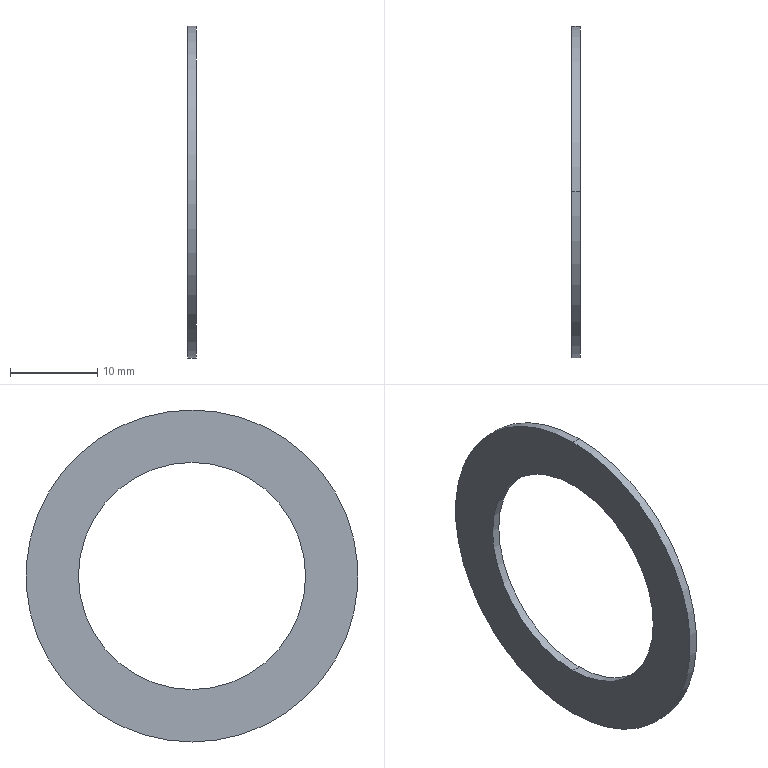Part | STEP file | 1 solid | 6 faces | box 1 x 38 x 38 mm | volume 603.186 mm3 | cylinder 4 | plane 2 | commonest cylinder face diameters 26 x2 38 x2
STEP:
#1=CARTESIAN_POINT('',(0.,0.,0.));
#2=DIRECTION('',(0.,0.,1.));
#3=DIRECTION('',(1.,0.,0.));
#4=AXIS2_PLACEMENT_3D('',#1,#2,#3);
#5=CARTESIAN_POINT('',(0.,0.,-13.));
#6=VERTEX_POINT('',#5);
#7=CARTESIAN_POINT('',(1.,0.,-13.));
#8=VERTEX_POINT('',#7);
#9=CARTESIAN_POINT('',(0.5,0.,-13.));
#10=DIRECTION('',(1.,0.,0.));
#11=VECTOR('',#10,1.);
#12=LINE('',#9,#11);
#13=CARTESIAN_POINT('',(0.5,0.,0.));
#14=DIRECTION('',(1.,0.,0.));
#15=DIRECTION('',(0.,0.,-1.));
#16=AXIS2_PLACEMENT_3D('',#13,#14,#15);
#17=CYLINDRICAL_SURFACE('',#16,13.);
#18=CARTESIAN_POINT('',(6.283,0.));
#19=DIRECTION('',(0.,1.));
#20=VECTOR('',#19,1.);
#21=LINE('',#18,#20);
#22=(GEOMETRIC_REPRESENTATION_CONTEXT(2)PARAMETRIC_REPRESENTATION_CONTEXT()REPRESENTATION_CONTEXT('',''));
#23=DEFINITIONAL_REPRESENTATION('',(#21),#22);
#24=PCURVE('',#17,#23);
#25=CARTESIAN_POINT('',(0.5,0.,0.));
#26=DIRECTION('',(1.,0.,0.));
#27=DIRECTION('',(0.,0.,-1.));
#28=AXIS2_PLACEMENT_3D('',#25,#26,#27);
#29=CYLINDRICAL_SURFACE('',#28,13.);
#30=CARTESIAN_POINT('',(0.,0.));
#31=DIRECTION('',(0.,1.));
#32=VECTOR('',#31,1.);
#33=LINE('',#30,#32);
#34=(GEOMETRIC_REPRESENTATION_CONTEXT(2)PARAMETRIC_REPRESENTATION_CONTEXT()REPRESENTATION_CONTEXT('',''));
#35=DEFINITIONAL_REPRESENTATION('',(#33),#34);
#36=PCURVE('',#29,#35);
#37=SURFACE_CURVE('',#12,(#24,#36),.PCURVE_S1.);
#38=EDGE_CURVE('',#6,#8,#37,.T.);
#39=ORIENTED_EDGE('',*,*,#38,.T.);
#40=CARTESIAN_POINT('',(1.,0.,13.));
#41=VERTEX_POINT('',#40);
#42=CARTESIAN_POINT('',(1.,0.,0.));
#43=DIRECTION('',(-1.,0.,0.));
#44=DIRECTION('',(0.,0.,-1.));
#45=AXIS2_PLACEMENT_3D('',#42,#43,#44);
#46=CIRCLE('',#45,13.);
#47=CARTESIAN_POINT('',(6.283,0.5));
#48=DIRECTION('',(-1.,0.));
#49=VECTOR('',#48,1.);
#50=LINE('',#47,#49);
#51=(GEOMETRIC_REPRESENTATION_CONTEXT(2)PARAMETRIC_REPRESENTATION_CONTEXT()REPRESENTATION_CONTEXT('',''));
#52=DEFINITIONAL_REPRESENTATION('',(#50),#51);
#53=PCURVE('',#17,#52);
#54=CARTESIAN_POINT('',(1.,16.,0.));
#55=DIRECTION('',(1.,0.,0.));
#56=DIRECTION('',(0.,0.,-1.));
#57=AXIS2_PLACEMENT_3D('',#54,#55,#56);
#58=PLANE('',#57);
#59=CARTESIAN_POINT('',(13.,-16.));
#60=CARTESIAN_POINT('',(13.,-38.517));
#61=CARTESIAN_POINT('',(-6.5,-27.258));
#62=CARTESIAN_POINT('',(-26.,-16.));
#63=CARTESIAN_POINT('',(-6.5,-4.742));
#64=CARTESIAN_POINT('',(13.,6.517));
#65=CARTESIAN_POINT('',(13.,-16.));
#66=(BOUNDED_CURVE()B_SPLINE_CURVE(2,(#59,#60,#61,#62,#63,#64,#65),.UNSPECIFIED.,.T.,.F.)B_SPLINE_CURVE_WITH_KNOTS((1,2,2,2,2,1),(-2.094,0.,2.094,4.189,6.283,8.378),.UNSPECIFIED.)CURVE()GEOMETRIC_REPRESENTATION_ITEM()RATIONAL_B_SPLINE_CURVE((1.,0.5,1.,0.5,1.,0.5,1.))REPRESENTATION_ITEM(''));
#67=(GEOMETRIC_REPRESENTATION_CONTEXT(2)PARAMETRIC_REPRESENTATION_CONTEXT()REPRESENTATION_CONTEXT('',''));
#68=DEFINITIONAL_REPRESENTATION('',(#66),#67);
#69=PCURVE('',#58,#68);
#70=SURFACE_CURVE('',#46,(#53,#69),.PCURVE_S1.);
#71=EDGE_CURVE('',#8,#41,#70,.T.);
#72=ORIENTED_EDGE('',*,*,#71,.T.);
#73=CARTESIAN_POINT('',(0.,0.,13.));
#74=VERTEX_POINT('',#73);
#75=CARTESIAN_POINT('',(0.5,0.,13.));
#76=DIRECTION('',(1.,0.,0.));
#77=VECTOR('',#76,1.);
#78=LINE('',#75,#77);
#79=CARTESIAN_POINT('',(3.142,0.));
#80=DIRECTION('',(0.,1.));
#81=VECTOR('',#80,1.);
#82=LINE('',#79,#81);
#83=(GEOMETRIC_REPRESENTATION_CONTEXT(2)PARAMETRIC_REPRESENTATION_CONTEXT()REPRESENTATION_CONTEXT('',''));
#84=DEFINITIONAL_REPRESENTATION('',(#82),#83);
#85=PCURVE('',#17,#84);
#86=CARTESIAN_POINT('',(3.142,0.));
#87=DIRECTION('',(0.,1.));
#88=VECTOR('',#87,1.);
#89=LINE('',#86,#88);
#90=(GEOMETRIC_REPRESENTATION_CONTEXT(2)PARAMETRIC_REPRESENTATION_CONTEXT()REPRESENTATION_CONTEXT('',''));
#91=DEFINITIONAL_REPRESENTATION('',(#89),#90);
#92=PCURVE('',#29,#91);
#93=SURFACE_CURVE('',#78,(#85,#92),.PCURVE_S1.);
#94=EDGE_CURVE('',#74,#41,#93,.T.);
#95=ORIENTED_EDGE('',*,*,#94,.F.);
#96=CARTESIAN_POINT('',(0.,0.,0.));
#97=DIRECTION('',(1.,0.,0.));
#98=DIRECTION('',(0.,0.,-1.));
#99=AXIS2_PLACEMENT_3D('',#96,#97,#98);
#100=CIRCLE('',#99,13.);
#101=CARTESIAN_POINT('',(0.,-0.5));
#102=DIRECTION('',(1.,0.));
#103=VECTOR('',#102,1.);
#104=LINE('',#101,#103);
#105=(GEOMETRIC_REPRESENTATION_CONTEXT(2)PARAMETRIC_REPRESENTATION_CONTEXT()REPRESENTATION_CONTEXT('',''));
#106=DEFINITIONAL_REPRESENTATION('',(#104),#105);
#107=PCURVE('',#17,#106);
#108=CARTESIAN_POINT('',(0.,16.,0.));
#109=DIRECTION('',(-1.,0.,0.));
#110=DIRECTION('',(0.,0.,1.));
#111=AXIS2_PLACEMENT_3D('',#108,#109,#110);
#112=PLANE('',#111);
#113=CARTESIAN_POINT('',(-13.,-16.));
#114=CARTESIAN_POINT('',(-13.,6.517));
#115=CARTESIAN_POINT('',(6.5,-4.742));
#116=CARTESIAN_POINT('',(26.,-16.));
#117=CARTESIAN_POINT('',(6.5,-27.258));
#118=CARTESIAN_POINT('',(-13.,-38.517));
#119=CARTESIAN_POINT('',(-13.,-16.));
#120=(BOUNDED_CURVE()B_SPLINE_CURVE(2,(#113,#114,#115,#116,#117,#118,#119),.UNSPECIFIED.,.T.,.F.)B_SPLINE_CURVE_WITH_KNOTS((1,2,2,2,2,1),(-2.094,0.,2.094,4.189,6.283,8.378),.UNSPECIFIED.)CURVE()GEOMETRIC_REPRESENTATION_ITEM()RATIONAL_B_SPLINE_CURVE((1.,0.5,1.,0.5,1.,0.5,1.))REPRESENTATION_ITEM(''));
#121=(GEOMETRIC_REPRESENTATION_CONTEXT(2)PARAMETRIC_REPRESENTATION_CONTEXT()REPRESENTATION_CONTEXT('',''));
#122=DEFINITIONAL_REPRESENTATION('',(#120),#121);
#123=PCURVE('',#112,#122);
#124=SURFACE_CURVE('',#100,(#107,#123),.PCURVE_S1.);
#125=EDGE_CURVE('',#74,#6,#124,.T.);
#126=ORIENTED_EDGE('',*,*,#125,.T.);
#127=EDGE_LOOP('',(#39,#72,#95,#126));
#128=FACE_BOUND('',#127,.F.);
#129=ADVANCED_FACE('',(#128),#17,.F.);
#130=CARTESIAN_POINT('',(0.,0.,-19.));
#131=VERTEX_POINT('',#130);
#132=CARTESIAN_POINT('',(0.,0.,19.));
#133=VERTEX_POINT('',#132);
#134=CARTESIAN_POINT('',(0.,0.,0.));
#135=DIRECTION('',(1.,0.,0.));
#136=DIRECTION('',(0.,0.,-1.));
#137=AXIS2_PLACEMENT_3D('',#134,#135,#136);
#138=CIRCLE('',#137,19.);
#139=CARTESIAN_POINT('',(0.5,0.,0.));
#140=DIRECTION('',(1.,0.,0.));
#141=DIRECTION('',(0.,0.,-1.));
#142=AXIS2_PLACEMENT_3D('',#139,#140,#141);
#143=CYLINDRICAL_SURFACE('',#142,19.);
#144=CARTESIAN_POINT('',(0.,-0.5));
#145=DIRECTION('',(1.,0.));
#146=VECTOR('',#145,1.);
#147=LINE('',#144,#146);
#148=(GEOMETRIC_REPRESENTATION_CONTEXT(2)PARAMETRIC_REPRESENTATION_CONTEXT()REPRESENTATION_CONTEXT('',''));
#149=DEFINITIONAL_REPRESENTATION('',(#147),#148);
#150=PCURVE('',#143,#149);
#151=CARTESIAN_POINT('',(-19.,-16.));
#152=CARTESIAN_POINT('',(-19.,16.909));
#153=CARTESIAN_POINT('',(9.5,0.4545));
#154=CARTESIAN_POINT('',(38.,-16.));
#155=CARTESIAN_POINT('',(9.5,-32.454));
#156=CARTESIAN_POINT('',(-19.,-48.909));
#157=CARTESIAN_POINT('',(-19.,-16.));
#158=(BOUNDED_CURVE()B_SPLINE_CURVE(2,(#151,#152,#153,#154,#155,#156,#157),.UNSPECIFIED.,.T.,.F.)B_SPLINE_CURVE_WITH_KNOTS((1,2,2,2,2,1),(-2.094,0.,2.094,4.189,6.283,8.378),.UNSPECIFIED.)CURVE()GEOMETRIC_REPRESENTATION_ITEM()RATIONAL_B_SPLINE_CURVE((1.,0.5,1.,0.5,1.,0.5,1.))REPRESENTATION_ITEM(''));
#159=(GEOMETRIC_REPRESENTATION_CONTEXT(2)PARAMETRIC_REPRESENTATION_CONTEXT()REPRESENTATION_CONTEXT('',''));
#160=DEFINITIONAL_REPRESENTATION('',(#158),#159);
#161=PCURVE('',#112,#160);
#162=SURFACE_CURVE('',#138,(#150,#161),.PCURVE_S1.);
#163=EDGE_CURVE('',#131,#133,#162,.T.);
#164=ORIENTED_EDGE('',*,*,#163,.T.);
#165=CARTESIAN_POINT('',(1.,0.,19.));
#166=VERTEX_POINT('',#165);
#167=CARTESIAN_POINT('',(0.5,0.,19.));
#168=DIRECTION('',(1.,0.,0.));
#169=VECTOR('',#168,1.);
#170=LINE('',#167,#169);
#171=CARTESIAN_POINT('',(3.142,0.));
#172=DIRECTION('',(0.,1.));
#173=VECTOR('',#172,1.);
#174=LINE('',#171,#173);
#175=(GEOMETRIC_REPRESENTATION_CONTEXT(2)PARAMETRIC_REPRESENTATION_CONTEXT()REPRESENTATION_CONTEXT('',''));
#176=DEFINITIONAL_REPRESENTATION('',(#174),#175);
#177=PCURVE('',#143,#176);
#178=CARTESIAN_POINT('',(0.5,0.,0.));
#179=DIRECTION('',(1.,0.,0.));
#180=DIRECTION('',(0.,0.,-1.));
#181=AXIS2_PLACEMENT_3D('',#178,#179,#180);
#182=CYLINDRICAL_SURFACE('',#181,19.);
#183=CARTESIAN_POINT('',(3.142,0.));
#184=DIRECTION('',(0.,1.));
#185=VECTOR('',#184,1.);
#186=LINE('',#183,#185);
#187=(GEOMETRIC_REPRESENTATION_CONTEXT(2)PARAMETRIC_REPRESENTATION_CONTEXT()REPRESENTATION_CONTEXT('',''));
#188=DEFINITIONAL_REPRESENTATION('',(#186),#187);
#189=PCURVE('',#182,#188);
#190=SURFACE_CURVE('',#170,(#177,#189),.PCURVE_S1.);
#191=EDGE_CURVE('',#133,#166,#190,.T.);
#192=ORIENTED_EDGE('',*,*,#191,.T.);
#193=CARTESIAN_POINT('',(1.,0.,-19.));
#194=VERTEX_POINT('',#193);
#195=CARTESIAN_POINT('',(1.,0.,0.));
#196=DIRECTION('',(1.,0.,0.));
#197=DIRECTION('',(0.,0.,-1.));
#198=AXIS2_PLACEMENT_3D('',#195,#196,#197);
#199=CIRCLE('',#198,19.);
#200=CARTESIAN_POINT('',(0.,0.5));
#201=DIRECTION('',(1.,0.));
#202=VECTOR('',#201,1.);
#203=LINE('',#200,#202);
#204=(GEOMETRIC_REPRESENTATION_CONTEXT(2)PARAMETRIC_REPRESENTATION_CONTEXT()REPRESENTATION_CONTEXT('',''));
#205=DEFINITIONAL_REPRESENTATION('',(#203),#204);
#206=PCURVE('',#143,#205);
#207=CARTESIAN_POINT('',(0.,-16.));
#208=DIRECTION('',(1.,0.));
#209=AXIS2_PLACEMENT_2D('',#207,#208);
#210=CIRCLE('',#209,19.);
#211=(GEOMETRIC_REPRESENTATION_CONTEXT(2)PARAMETRIC_REPRESENTATION_CONTEXT()REPRESENTATION_CONTEXT('',''));
#212=DEFINITIONAL_REPRESENTATION('',(#210),#211);
#213=PCURVE('',#58,#212);
#214=SURFACE_CURVE('',#199,(#206,#213),.PCURVE_S1.);
#215=EDGE_CURVE('',#194,#166,#214,.T.);
#216=ORIENTED_EDGE('',*,*,#215,.F.);
#217=CARTESIAN_POINT('',(0.5,0.,-19.));
#218=DIRECTION('',(1.,0.,0.));
#219=VECTOR('',#218,1.);
#220=LINE('',#217,#219);
#221=CARTESIAN_POINT('',(0.,0.));
#222=DIRECTION('',(0.,1.));
#223=VECTOR('',#222,1.);
#224=LINE('',#221,#223);
#225=(GEOMETRIC_REPRESENTATION_CONTEXT(2)PARAMETRIC_REPRESENTATION_CONTEXT()REPRESENTATION_CONTEXT('',''));
#226=DEFINITIONAL_REPRESENTATION('',(#224),#225);
#227=PCURVE('',#143,#226);
#228=CARTESIAN_POINT('',(6.283,0.));
#229=DIRECTION('',(0.,1.));
#230=VECTOR('',#229,1.);
#231=LINE('',#228,#230);
#232=(GEOMETRIC_REPRESENTATION_CONTEXT(2)PARAMETRIC_REPRESENTATION_CONTEXT()REPRESENTATION_CONTEXT('',''));
#233=DEFINITIONAL_REPRESENTATION('',(#231),#232);
#234=PCURVE('',#182,#233);
#235=SURFACE_CURVE('',#220,(#227,#234),.PCURVE_S1.);
#236=EDGE_CURVE('',#131,#194,#235,.T.);
#237=ORIENTED_EDGE('',*,*,#236,.F.);
#238=EDGE_LOOP('',(#164,#192,#216,#237));
#239=FACE_BOUND('',#238,.T.);
#240=ADVANCED_FACE('',(#239),#143,.T.);
#241=ORIENTED_EDGE('',*,*,#71,.T.);
#242=CARTESIAN_POINT('',(1.,0.,0.));
#243=DIRECTION('',(-1.,0.,0.));
#244=DIRECTION('',(0.,0.,-1.));
#245=AXIS2_PLACEMENT_3D('',#242,#243,#244);
#246=CIRCLE('',#245,13.);
#247=CARTESIAN_POINT('',(13.,-16.));
#248=CARTESIAN_POINT('',(13.,-38.517));
#249=CARTESIAN_POINT('',(-6.5,-27.258));
#250=CARTESIAN_POINT('',(-26.,-16.));
#251=CARTESIAN_POINT('',(-6.5,-4.742));
#252=CARTESIAN_POINT('',(13.,6.517));
#253=CARTESIAN_POINT('',(13.,-16.));
#254=(BOUNDED_CURVE()B_SPLINE_CURVE(2,(#247,#248,#249,#250,#251,#252,#253),.UNSPECIFIED.,.T.,.F.)B_SPLINE_CURVE_WITH_KNOTS((1,2,2,2,2,1),(-2.094,0.,2.094,4.189,6.283,8.378),.UNSPECIFIED.)CURVE()GEOMETRIC_REPRESENTATION_ITEM()RATIONAL_B_SPLINE_CURVE((1.,0.5,1.,0.5,1.,0.5,1.))REPRESENTATION_ITEM(''));
#255=(GEOMETRIC_REPRESENTATION_CONTEXT(2)PARAMETRIC_REPRESENTATION_CONTEXT()REPRESENTATION_CONTEXT('',''));
#256=DEFINITIONAL_REPRESENTATION('',(#254),#255);
#257=PCURVE('',#58,#256);
#258=CARTESIAN_POINT('',(6.283,0.5));
#259=DIRECTION('',(-1.,0.));
#260=VECTOR('',#259,1.);
#261=LINE('',#258,#260);
#262=(GEOMETRIC_REPRESENTATION_CONTEXT(2)PARAMETRIC_REPRESENTATION_CONTEXT()REPRESENTATION_CONTEXT('',''));
#263=DEFINITIONAL_REPRESENTATION('',(#261),#262);
#264=PCURVE('',#29,#263);
#265=SURFACE_CURVE('',#246,(#257,#264),.PCURVE_S1.);
#266=EDGE_CURVE('',#41,#8,#265,.T.);
#267=ORIENTED_EDGE('',*,*,#266,.T.);
#268=EDGE_LOOP('',(#241,#267));
#269=FACE_BOUND('',#268,.T.);
#270=ORIENTED_EDGE('',*,*,#215,.T.);
#271=CARTESIAN_POINT('',(1.,0.,0.));
#272=DIRECTION('',(1.,0.,0.));
#273=DIRECTION('',(0.,0.,-1.));
#274=AXIS2_PLACEMENT_3D('',#271,#272,#273);
#275=CIRCLE('',#274,19.);
#276=CARTESIAN_POINT('',(0.,-16.));
#277=DIRECTION('',(1.,0.));
#278=AXIS2_PLACEMENT_2D('',#276,#277);
#279=CIRCLE('',#278,19.);
#280=(GEOMETRIC_REPRESENTATION_CONTEXT(2)PARAMETRIC_REPRESENTATION_CONTEXT()REPRESENTATION_CONTEXT('',''));
#281=DEFINITIONAL_REPRESENTATION('',(#279),#280);
#282=PCURVE('',#58,#281);
#283=CARTESIAN_POINT('',(0.,0.5));
#284=DIRECTION('',(1.,0.));
#285=VECTOR('',#284,1.);
#286=LINE('',#283,#285);
#287=(GEOMETRIC_REPRESENTATION_CONTEXT(2)PARAMETRIC_REPRESENTATION_CONTEXT()REPRESENTATION_CONTEXT('',''));
#288=DEFINITIONAL_REPRESENTATION('',(#286),#287);
#289=PCURVE('',#182,#288);
#290=SURFACE_CURVE('',#275,(#282,#289),.PCURVE_S1.);
#291=EDGE_CURVE('',#166,#194,#290,.T.);
#292=ORIENTED_EDGE('',*,*,#291,.T.);
#293=EDGE_LOOP('',(#270,#292));
#294=FACE_BOUND('',#293,.T.);
#295=ADVANCED_FACE('',(#269,#294),#58,.T.);
#296=ORIENTED_EDGE('',*,*,#266,.T.);
#297=ORIENTED_EDGE('',*,*,#38,.F.);
#298=CARTESIAN_POINT('',(0.,0.,0.));
#299=DIRECTION('',(1.,0.,0.));
#300=DIRECTION('',(0.,0.,-1.));
#301=AXIS2_PLACEMENT_3D('',#298,#299,#300);
#302=CIRCLE('',#301,13.);
#303=CARTESIAN_POINT('',(0.,-0.5));
#304=DIRECTION('',(1.,0.));
#305=VECTOR('',#304,1.);
#306=LINE('',#303,#305);
#307=(GEOMETRIC_REPRESENTATION_CONTEXT(2)PARAMETRIC_REPRESENTATION_CONTEXT()REPRESENTATION_CONTEXT('',''));
#308=DEFINITIONAL_REPRESENTATION('',(#306),#307);
#309=PCURVE('',#29,#308);
#310=CARTESIAN_POINT('',(-13.,-16.));
#311=CARTESIAN_POINT('',(-13.,6.517));
#312=CARTESIAN_POINT('',(6.5,-4.742));
#313=CARTESIAN_POINT('',(26.,-16.));
#314=CARTESIAN_POINT('',(6.5,-27.258));
#315=CARTESIAN_POINT('',(-13.,-38.517));
#316=CARTESIAN_POINT('',(-13.,-16.));
#317=(BOUNDED_CURVE()B_SPLINE_CURVE(2,(#310,#311,#312,#313,#314,#315,#316),.UNSPECIFIED.,.T.,.F.)B_SPLINE_CURVE_WITH_KNOTS((1,2,2,2,2,1),(-2.094,0.,2.094,4.189,6.283,8.378),.UNSPECIFIED.)CURVE()GEOMETRIC_REPRESENTATION_ITEM()RATIONAL_B_SPLINE_CURVE((1.,0.5,1.,0.5,1.,0.5,1.))REPRESENTATION_ITEM(''));
#318=(GEOMETRIC_REPRESENTATION_CONTEXT(2)PARAMETRIC_REPRESENTATION_CONTEXT()REPRESENTATION_CONTEXT('',''));
#319=DEFINITIONAL_REPRESENTATION('',(#317),#318);
#320=PCURVE('',#112,#319);
#321=SURFACE_CURVE('',#302,(#309,#320),.PCURVE_S1.);
#322=EDGE_CURVE('',#6,#74,#321,.T.);
#323=ORIENTED_EDGE('',*,*,#322,.T.);
#324=ORIENTED_EDGE('',*,*,#94,.T.);
#325=EDGE_LOOP('',(#296,#297,#323,#324));
#326=FACE_BOUND('',#325,.F.);
#327=ADVANCED_FACE('',(#326),#29,.F.);
#328=ORIENTED_EDGE('',*,*,#191,.F.);
#329=CARTESIAN_POINT('',(0.,0.,0.));
#330=DIRECTION('',(1.,0.,0.));
#331=DIRECTION('',(0.,0.,-1.));
#332=AXIS2_PLACEMENT_3D('',#329,#330,#331);
#333=CIRCLE('',#332,19.);
#334=CARTESIAN_POINT('',(0.,-0.5));
#335=DIRECTION('',(1.,0.));
#336=VECTOR('',#335,1.);
#337=LINE('',#334,#336);
#338=(GEOMETRIC_REPRESENTATION_CONTEXT(2)PARAMETRIC_REPRESENTATION_CONTEXT()REPRESENTATION_CONTEXT('',''));
#339=DEFINITIONAL_REPRESENTATION('',(#337),#338);
#340=PCURVE('',#182,#339);
#341=CARTESIAN_POINT('',(-19.,-16.));
#342=CARTESIAN_POINT('',(-19.,16.909));
#343=CARTESIAN_POINT('',(9.5,0.4545));
#344=CARTESIAN_POINT('',(38.,-16.));
#345=CARTESIAN_POINT('',(9.5,-32.454));
#346=CARTESIAN_POINT('',(-19.,-48.909));
#347=CARTESIAN_POINT('',(-19.,-16.));
#348=(BOUNDED_CURVE()B_SPLINE_CURVE(2,(#341,#342,#343,#344,#345,#346,#347),.UNSPECIFIED.,.T.,.F.)B_SPLINE_CURVE_WITH_KNOTS((1,2,2,2,2,1),(-2.094,0.,2.094,4.189,6.283,8.378),.UNSPECIFIED.)CURVE()GEOMETRIC_REPRESENTATION_ITEM()RATIONAL_B_SPLINE_CURVE((1.,0.5,1.,0.5,1.,0.5,1.))REPRESENTATION_ITEM(''));
#349=(GEOMETRIC_REPRESENTATION_CONTEXT(2)PARAMETRIC_REPRESENTATION_CONTEXT()REPRESENTATION_CONTEXT('',''));
#350=DEFINITIONAL_REPRESENTATION('',(#348),#349);
#351=PCURVE('',#112,#350);
#352=SURFACE_CURVE('',#333,(#340,#351),.PCURVE_S1.);
#353=EDGE_CURVE('',#133,#131,#352,.T.);
#354=ORIENTED_EDGE('',*,*,#353,.T.);
#355=ORIENTED_EDGE('',*,*,#236,.T.);
#356=ORIENTED_EDGE('',*,*,#291,.F.);
#357=EDGE_LOOP('',(#328,#354,#355,#356));
#358=FACE_BOUND('',#357,.T.);
#359=ADVANCED_FACE('',(#358),#182,.T.);
#360=ORIENTED_EDGE('',*,*,#322,.T.);
#361=ORIENTED_EDGE('',*,*,#125,.T.);
#362=EDGE_LOOP('',(#360,#361));
#363=FACE_BOUND('',#362,.T.);
#364=ORIENTED_EDGE('',*,*,#163,.F.);
#365=ORIENTED_EDGE('',*,*,#353,.F.);
#366=EDGE_LOOP('',(#364,#365));
#367=FACE_BOUND('',#366,.T.);
#368=ADVANCED_FACE('',(#363,#367),#112,.T.);
#369=CLOSED_SHELL('',(#129,#240,#295,#327,#359,#368));
#370=MANIFOLD_SOLID_BREP('',#369);
#371=(LENGTH_UNIT()NAMED_UNIT(*)SI_UNIT(.MILLI.,.METRE.));
#372=UNCERTAINTY_MEASURE_WITH_UNIT(LENGTH_MEASURE(0.0000001),#371,'','');
#373=(NAMED_UNIT(*)PLANE_ANGLE_UNIT()SI_UNIT($,.RADIAN.));
#374=(NAMED_UNIT(*)SI_UNIT($,.STERADIAN.)SOLID_ANGLE_UNIT());
#375=(GEOMETRIC_REPRESENTATION_CONTEXT(3)GLOBAL_UNCERTAINTY_ASSIGNED_CONTEXT((#372))GLOBAL_UNIT_ASSIGNED_CONTEXT((#371,#373,#374))REPRESENTATION_CONTEXT('',''));
#376=ADVANCED_BREP_SHAPE_REPRESENTATION('',(#4,#370),#375);